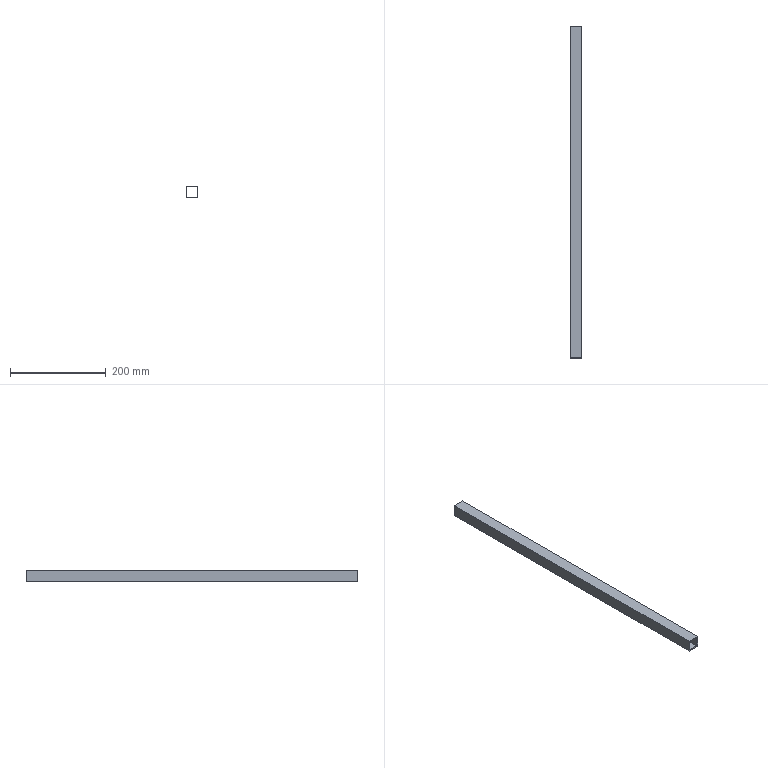Part | NX | features solid 2 | 1 solid | 10 faces | box 25 x 695 x 25 mm | volume 127880 mm3 | plane 10
STEP:
#1=CARTESIAN_POINT('',(300.,347.5,35.));
#2=VERTEX_POINT('',#1);
#3=CARTESIAN_POINT('',(325.,347.5,35.));
#4=VERTEX_POINT('',#3);
#5=CARTESIAN_POINT('',(137.5,347.5,35.));
#6=DIRECTION('',(-1.,0.,0.));
#7=VECTOR('',#6,1000.);
#8=LINE('',#5,#7);
#9=EDGE_CURVE('',#2,#4,#8,.F.);
#10=ORIENTED_EDGE('',*,*,#9,.T.);
#11=CARTESIAN_POINT('',(325.,347.5,10.));
#12=VERTEX_POINT('',#11);
#13=CARTESIAN_POINT('',(325.,347.5,15.));
#14=DIRECTION('',(0.,0.,1.));
#15=VECTOR('',#14,1000.);
#16=LINE('',#13,#15);
#17=EDGE_CURVE('',#12,#4,#16,.T.);
#18=ORIENTED_EDGE('',*,*,#17,.F.);
#19=CARTESIAN_POINT('',(300.,347.5,10.));
#20=VERTEX_POINT('',#19);
#21=CARTESIAN_POINT('',(445.,347.5,10.));
#22=DIRECTION('',(1.,0.,0.));
#23=VECTOR('',#22,1000.);
#24=LINE('',#21,#23);
#25=EDGE_CURVE('',#20,#12,#24,.T.);
#26=ORIENTED_EDGE('',*,*,#25,.F.);
#27=CARTESIAN_POINT('',(300.,347.5,15.));
#28=DIRECTION('',(0.,0.,1.));
#29=VECTOR('',#28,1000.);
#30=LINE('',#27,#29);
#31=EDGE_CURVE('',#20,#2,#30,.T.);
#32=ORIENTED_EDGE('',*,*,#31,.T.);
#33=EDGE_LOOP('',(#10,#18,#26,#32));
#34=FACE_BOUND('',#33,.T.);
#35=CARTESIAN_POINT('',(302.,347.5,33.));
#36=VERTEX_POINT('',#35);
#37=CARTESIAN_POINT('',(323.,347.5,33.));
#38=VERTEX_POINT('',#37);
#39=CARTESIAN_POINT('',(137.5,347.5,33.));
#40=DIRECTION('',(-1.,0.,0.));
#41=VECTOR('',#40,1000.);
#42=LINE('',#39,#41);
#43=EDGE_CURVE('',#36,#38,#42,.F.);
#44=ORIENTED_EDGE('',*,*,#43,.F.);
#45=CARTESIAN_POINT('',(302.,347.5,12.));
#46=VERTEX_POINT('',#45);
#47=CARTESIAN_POINT('',(302.,347.5,15.));
#48=DIRECTION('',(0.,0.,1.));
#49=VECTOR('',#48,1000.);
#50=LINE('',#47,#49);
#51=EDGE_CURVE('',#46,#36,#50,.T.);
#52=ORIENTED_EDGE('',*,*,#51,.F.);
#53=CARTESIAN_POINT('',(323.,347.5,12.));
#54=VERTEX_POINT('',#53);
#55=CARTESIAN_POINT('',(445.,347.5,12.));
#56=DIRECTION('',(1.,0.,0.));
#57=VECTOR('',#56,1000.);
#58=LINE('',#55,#57);
#59=EDGE_CURVE('',#46,#54,#58,.T.);
#60=ORIENTED_EDGE('',*,*,#59,.T.);
#61=CARTESIAN_POINT('',(323.,347.5,15.));
#62=DIRECTION('',(0.,0.,1.));
#63=VECTOR('',#62,1000.);
#64=LINE('',#61,#63);
#65=EDGE_CURVE('',#54,#38,#64,.T.);
#66=ORIENTED_EDGE('',*,*,#65,.T.);
#67=EDGE_LOOP('',(#44,#52,#60,#66));
#68=FACE_BOUND('',#67,.T.);
#69=CARTESIAN_POINT('',(137.5,347.5,15.));
#70=DIRECTION('',(0.,-1.,0.));
#71=DIRECTION('',(0.,0.,-1.));
#72=AXIS2_PLACEMENT_3D('',#69,#70,#71);
#73=PLANE('',#72);
#74=ADVANCED_FACE('',(#34,#68),#73,.F.);
#75=ORIENTED_EDGE('',*,*,#25,.T.);
#76=CARTESIAN_POINT('',(325.,-347.5,10.));
#77=VERTEX_POINT('',#76);
#78=CARTESIAN_POINT('',(325.,537.5,10.));
#79=DIRECTION('',(0.,-1.,0.));
#80=VECTOR('',#79,1000.);
#81=LINE('',#78,#80);
#82=EDGE_CURVE('',#12,#77,#81,.T.);
#83=ORIENTED_EDGE('',*,*,#82,.T.);
#84=CARTESIAN_POINT('',(300.,-347.5,10.));
#85=VERTEX_POINT('',#84);
#86=CARTESIAN_POINT('',(137.5,-347.5,10.));
#87=DIRECTION('',(1.,0.,0.));
#88=VECTOR('',#87,1000.);
#89=LINE('',#86,#88);
#90=EDGE_CURVE('',#85,#77,#89,.T.);
#91=ORIENTED_EDGE('',*,*,#90,.F.);
#92=CARTESIAN_POINT('',(300.,537.5,10.));
#93=DIRECTION('',(0.,-1.,0.));
#94=VECTOR('',#93,1000.);
#95=LINE('',#92,#94);
#96=EDGE_CURVE('',#20,#85,#95,.T.);
#97=ORIENTED_EDGE('',*,*,#96,.F.);
#98=EDGE_LOOP('',(#75,#83,#91,#97));
#99=FACE_BOUND('',#98,.T.);
#100=CARTESIAN_POINT('',(445.,537.5,10.));
#101=DIRECTION('',(0.,0.,1.));
#102=DIRECTION('',(0.,-1.,0.));
#103=AXIS2_PLACEMENT_3D('',#100,#101,#102);
#104=PLANE('',#103);
#105=ADVANCED_FACE('',(#99),#104,.F.);
#106=CARTESIAN_POINT('',(300.,-347.5,35.));
#107=VERTEX_POINT('',#106);
#108=CARTESIAN_POINT('',(300.,537.5,35.));
#109=DIRECTION('',(0.,1.,0.));
#110=VECTOR('',#109,1000.);
#111=LINE('',#108,#110);
#112=EDGE_CURVE('',#2,#107,#111,.F.);
#113=ORIENTED_EDGE('',*,*,#112,.T.);
#114=CARTESIAN_POINT('',(325.,-347.5,35.));
#115=VERTEX_POINT('',#114);
#116=CARTESIAN_POINT('',(445.,-347.5,35.));
#117=DIRECTION('',(-1.,0.,0.));
#118=VECTOR('',#117,1000.);
#119=LINE('',#116,#118);
#120=EDGE_CURVE('',#107,#115,#119,.F.);
#121=ORIENTED_EDGE('',*,*,#120,.T.);
#122=CARTESIAN_POINT('',(325.,537.5,35.));
#123=DIRECTION('',(0.,1.,0.));
#124=VECTOR('',#123,1000.);
#125=LINE('',#122,#124);
#126=EDGE_CURVE('',#4,#115,#125,.F.);
#127=ORIENTED_EDGE('',*,*,#126,.F.);
#128=ORIENTED_EDGE('',*,*,#9,.F.);
#129=EDGE_LOOP('',(#113,#121,#127,#128));
#130=FACE_BOUND('',#129,.T.);
#131=CARTESIAN_POINT('',(445.,537.5,35.));
#132=DIRECTION('',(0.,0.,1.));
#133=DIRECTION('',(0.,-1.,0.));
#134=AXIS2_PLACEMENT_3D('',#131,#132,#133);
#135=PLANE('',#134);
#136=ADVANCED_FACE('',(#130),#135,.T.);
#137=ORIENTED_EDGE('',*,*,#126,.T.);
#138=CARTESIAN_POINT('',(325.,-347.5,20.));
#139=DIRECTION('',(0.,0.,1.));
#140=VECTOR('',#139,1000.);
#141=LINE('',#138,#140);
#142=EDGE_CURVE('',#77,#115,#141,.T.);
#143=ORIENTED_EDGE('',*,*,#142,.F.);
#144=ORIENTED_EDGE('',*,*,#82,.F.);
#145=ORIENTED_EDGE('',*,*,#17,.T.);
#146=EDGE_LOOP('',(#137,#143,#144,#145));
#147=FACE_BOUND('',#146,.T.);
#148=CARTESIAN_POINT('',(325.,537.5,20.));
#149=DIRECTION('',(1.,0.,0.));
#150=DIRECTION('',(0.,0.,-1.));
#151=AXIS2_PLACEMENT_3D('',#148,#149,#150);
#152=PLANE('',#151);
#153=ADVANCED_FACE('',(#147),#152,.T.);
#154=ORIENTED_EDGE('',*,*,#96,.T.);
#155=CARTESIAN_POINT('',(300.,-347.5,20.));
#156=DIRECTION('',(0.,0.,1.));
#157=VECTOR('',#156,1000.);
#158=LINE('',#155,#157);
#159=EDGE_CURVE('',#85,#107,#158,.T.);
#160=ORIENTED_EDGE('',*,*,#159,.T.);
#161=ORIENTED_EDGE('',*,*,#112,.F.);
#162=ORIENTED_EDGE('',*,*,#31,.F.);
#163=EDGE_LOOP('',(#154,#160,#161,#162));
#164=FACE_BOUND('',#163,.T.);
#165=CARTESIAN_POINT('',(300.,537.5,20.));
#166=DIRECTION('',(1.,0.,0.));
#167=DIRECTION('',(0.,0.,-1.));
#168=AXIS2_PLACEMENT_3D('',#165,#166,#167);
#169=PLANE('',#168);
#170=ADVANCED_FACE('',(#164),#169,.F.);
#171=CARTESIAN_POINT('',(323.,-347.5,12.));
#172=VERTEX_POINT('',#171);
#173=CARTESIAN_POINT('',(323.,537.5,12.));
#174=DIRECTION('',(0.,-1.,0.));
#175=VECTOR('',#174,1000.);
#176=LINE('',#173,#175);
#177=EDGE_CURVE('',#54,#172,#176,.T.);
#178=ORIENTED_EDGE('',*,*,#177,.F.);
#179=ORIENTED_EDGE('',*,*,#59,.F.);
#180=CARTESIAN_POINT('',(302.,-347.5,12.));
#181=VERTEX_POINT('',#180);
#182=CARTESIAN_POINT('',(302.,537.5,12.));
#183=DIRECTION('',(0.,-1.,0.));
#184=VECTOR('',#183,1000.);
#185=LINE('',#182,#184);
#186=EDGE_CURVE('',#46,#181,#185,.T.);
#187=ORIENTED_EDGE('',*,*,#186,.T.);
#188=CARTESIAN_POINT('',(137.5,-347.5,12.));
#189=DIRECTION('',(1.,0.,0.));
#190=VECTOR('',#189,1000.);
#191=LINE('',#188,#190);
#192=EDGE_CURVE('',#181,#172,#191,.T.);
#193=ORIENTED_EDGE('',*,*,#192,.T.);
#194=EDGE_LOOP('',(#178,#179,#187,#193));
#195=FACE_BOUND('',#194,.T.);
#196=CARTESIAN_POINT('',(445.,537.5,12.));
#197=DIRECTION('',(0.,0.,1.));
#198=DIRECTION('',(0.,-1.,0.));
#199=AXIS2_PLACEMENT_3D('',#196,#197,#198);
#200=PLANE('',#199);
#201=ADVANCED_FACE('',(#195),#200,.T.);
#202=CARTESIAN_POINT('',(302.,-347.5,33.));
#203=VERTEX_POINT('',#202);
#204=CARTESIAN_POINT('',(302.,537.5,33.));
#205=DIRECTION('',(0.,1.,0.));
#206=VECTOR('',#205,1000.);
#207=LINE('',#204,#206);
#208=EDGE_CURVE('',#36,#203,#207,.F.);
#209=ORIENTED_EDGE('',*,*,#208,.F.);
#210=ORIENTED_EDGE('',*,*,#43,.T.);
#211=CARTESIAN_POINT('',(323.,-347.5,33.));
#212=VERTEX_POINT('',#211);
#213=CARTESIAN_POINT('',(323.,537.5,33.));
#214=DIRECTION('',(0.,1.,0.));
#215=VECTOR('',#214,1000.);
#216=LINE('',#213,#215);
#217=EDGE_CURVE('',#38,#212,#216,.F.);
#218=ORIENTED_EDGE('',*,*,#217,.T.);
#219=CARTESIAN_POINT('',(445.,-347.5,33.));
#220=DIRECTION('',(-1.,0.,0.));
#221=VECTOR('',#220,1000.);
#222=LINE('',#219,#221);
#223=EDGE_CURVE('',#203,#212,#222,.F.);
#224=ORIENTED_EDGE('',*,*,#223,.F.);
#225=EDGE_LOOP('',(#209,#210,#218,#224));
#226=FACE_BOUND('',#225,.T.);
#227=CARTESIAN_POINT('',(445.,537.5,33.));
#228=DIRECTION('',(0.,0.,1.));
#229=DIRECTION('',(0.,-1.,0.));
#230=AXIS2_PLACEMENT_3D('',#227,#228,#229);
#231=PLANE('',#230);
#232=ADVANCED_FACE('',(#226),#231,.F.);
#233=ORIENTED_EDGE('',*,*,#177,.T.);
#234=CARTESIAN_POINT('',(323.,-347.5,20.));
#235=DIRECTION('',(0.,0.,1.));
#236=VECTOR('',#235,1000.);
#237=LINE('',#234,#236);
#238=EDGE_CURVE('',#172,#212,#237,.T.);
#239=ORIENTED_EDGE('',*,*,#238,.T.);
#240=ORIENTED_EDGE('',*,*,#217,.F.);
#241=ORIENTED_EDGE('',*,*,#65,.F.);
#242=EDGE_LOOP('',(#233,#239,#240,#241));
#243=FACE_BOUND('',#242,.T.);
#244=CARTESIAN_POINT('',(323.,537.5,20.));
#245=DIRECTION('',(1.,0.,0.));
#246=DIRECTION('',(0.,0.,-1.));
#247=AXIS2_PLACEMENT_3D('',#244,#245,#246);
#248=PLANE('',#247);
#249=ADVANCED_FACE('',(#243),#248,.F.);
#250=ORIENTED_EDGE('',*,*,#208,.T.);
#251=CARTESIAN_POINT('',(302.,-347.5,20.));
#252=DIRECTION('',(0.,0.,1.));
#253=VECTOR('',#252,1000.);
#254=LINE('',#251,#253);
#255=EDGE_CURVE('',#181,#203,#254,.T.);
#256=ORIENTED_EDGE('',*,*,#255,.F.);
#257=ORIENTED_EDGE('',*,*,#186,.F.);
#258=ORIENTED_EDGE('',*,*,#51,.T.);
#259=EDGE_LOOP('',(#250,#256,#257,#258));
#260=FACE_BOUND('',#259,.T.);
#261=CARTESIAN_POINT('',(302.,537.5,20.));
#262=DIRECTION('',(1.,0.,0.));
#263=DIRECTION('',(0.,0.,-1.));
#264=AXIS2_PLACEMENT_3D('',#261,#262,#263);
#265=PLANE('',#264);
#266=ADVANCED_FACE('',(#260),#265,.T.);
#267=ORIENTED_EDGE('',*,*,#255,.T.);
#268=ORIENTED_EDGE('',*,*,#223,.T.);
#269=ORIENTED_EDGE('',*,*,#238,.F.);
#270=ORIENTED_EDGE('',*,*,#192,.F.);
#271=EDGE_LOOP('',(#267,#268,#269,#270));
#272=FACE_BOUND('',#271,.T.);
#273=ORIENTED_EDGE('',*,*,#120,.F.);
#274=ORIENTED_EDGE('',*,*,#159,.F.);
#275=ORIENTED_EDGE('',*,*,#90,.T.);
#276=ORIENTED_EDGE('',*,*,#142,.T.);
#277=EDGE_LOOP('',(#273,#274,#275,#276));
#278=FACE_BOUND('',#277,.T.);
#279=CARTESIAN_POINT('',(137.5,-347.5,15.));
#280=DIRECTION('',(0.,1.,0.));
#281=DIRECTION('',(0.,0.,-1.));
#282=AXIS2_PLACEMENT_3D('',#279,#280,#281);
#283=PLANE('',#282);
#284=ADVANCED_FACE('',(#272,#278),#283,.F.);
#285=CLOSED_SHELL('',(#74,#105,#136,#153,#170,#201,#232,#249,#266,#284));
#286=MANIFOLD_SOLID_BREP('',#285);
#287=(LENGTH_UNIT()NAMED_UNIT(*)SI_UNIT(.MILLI.,.METRE.));
#288=UNCERTAINTY_MEASURE_WITH_UNIT(LENGTH_MEASURE(0.00001),#287,'','');
#289=(NAMED_UNIT(*)PLANE_ANGLE_UNIT()SI_UNIT($,.RADIAN.));
#290=(NAMED_UNIT(*)SI_UNIT($,.STERADIAN.)SOLID_ANGLE_UNIT());
#291=(GEOMETRIC_REPRESENTATION_CONTEXT(3)GLOBAL_UNCERTAINTY_ASSIGNED_CONTEXT((#288))GLOBAL_UNIT_ASSIGNED_CONTEXT((#287,#289,#290))REPRESENTATION_CONTEXT('',''));
#292=ADVANCED_BREP_SHAPE_REPRESENTATION('',(#286),#291);